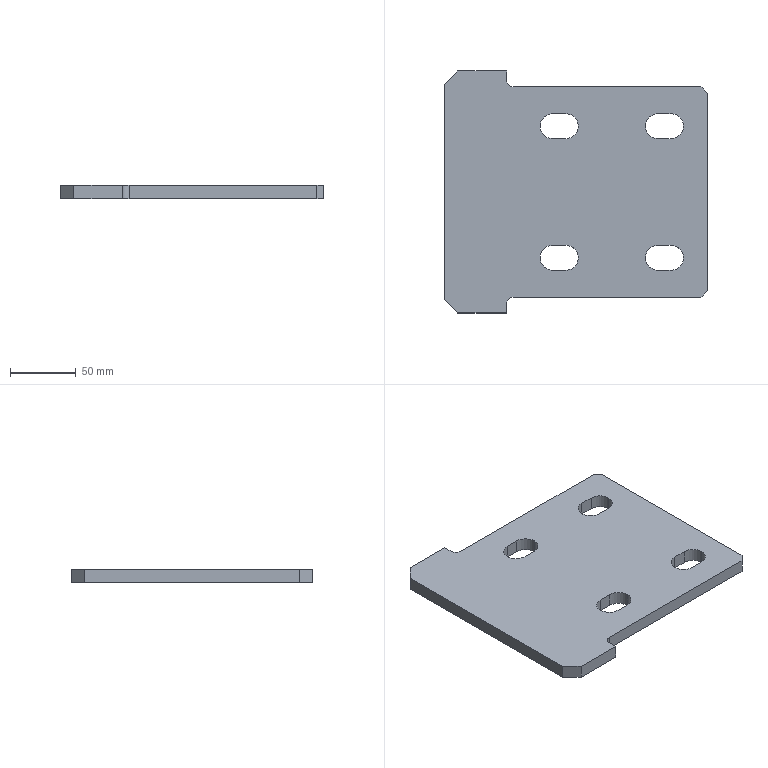Part | STEP file | 筋Plate 200-200 | 1 solid | 36 faces | box 200 x 184 x 10 mm | volume 311256 mm3 | plane 22 | cylinder 14 | commonest cylinder face diameters 19 x12 10 x2